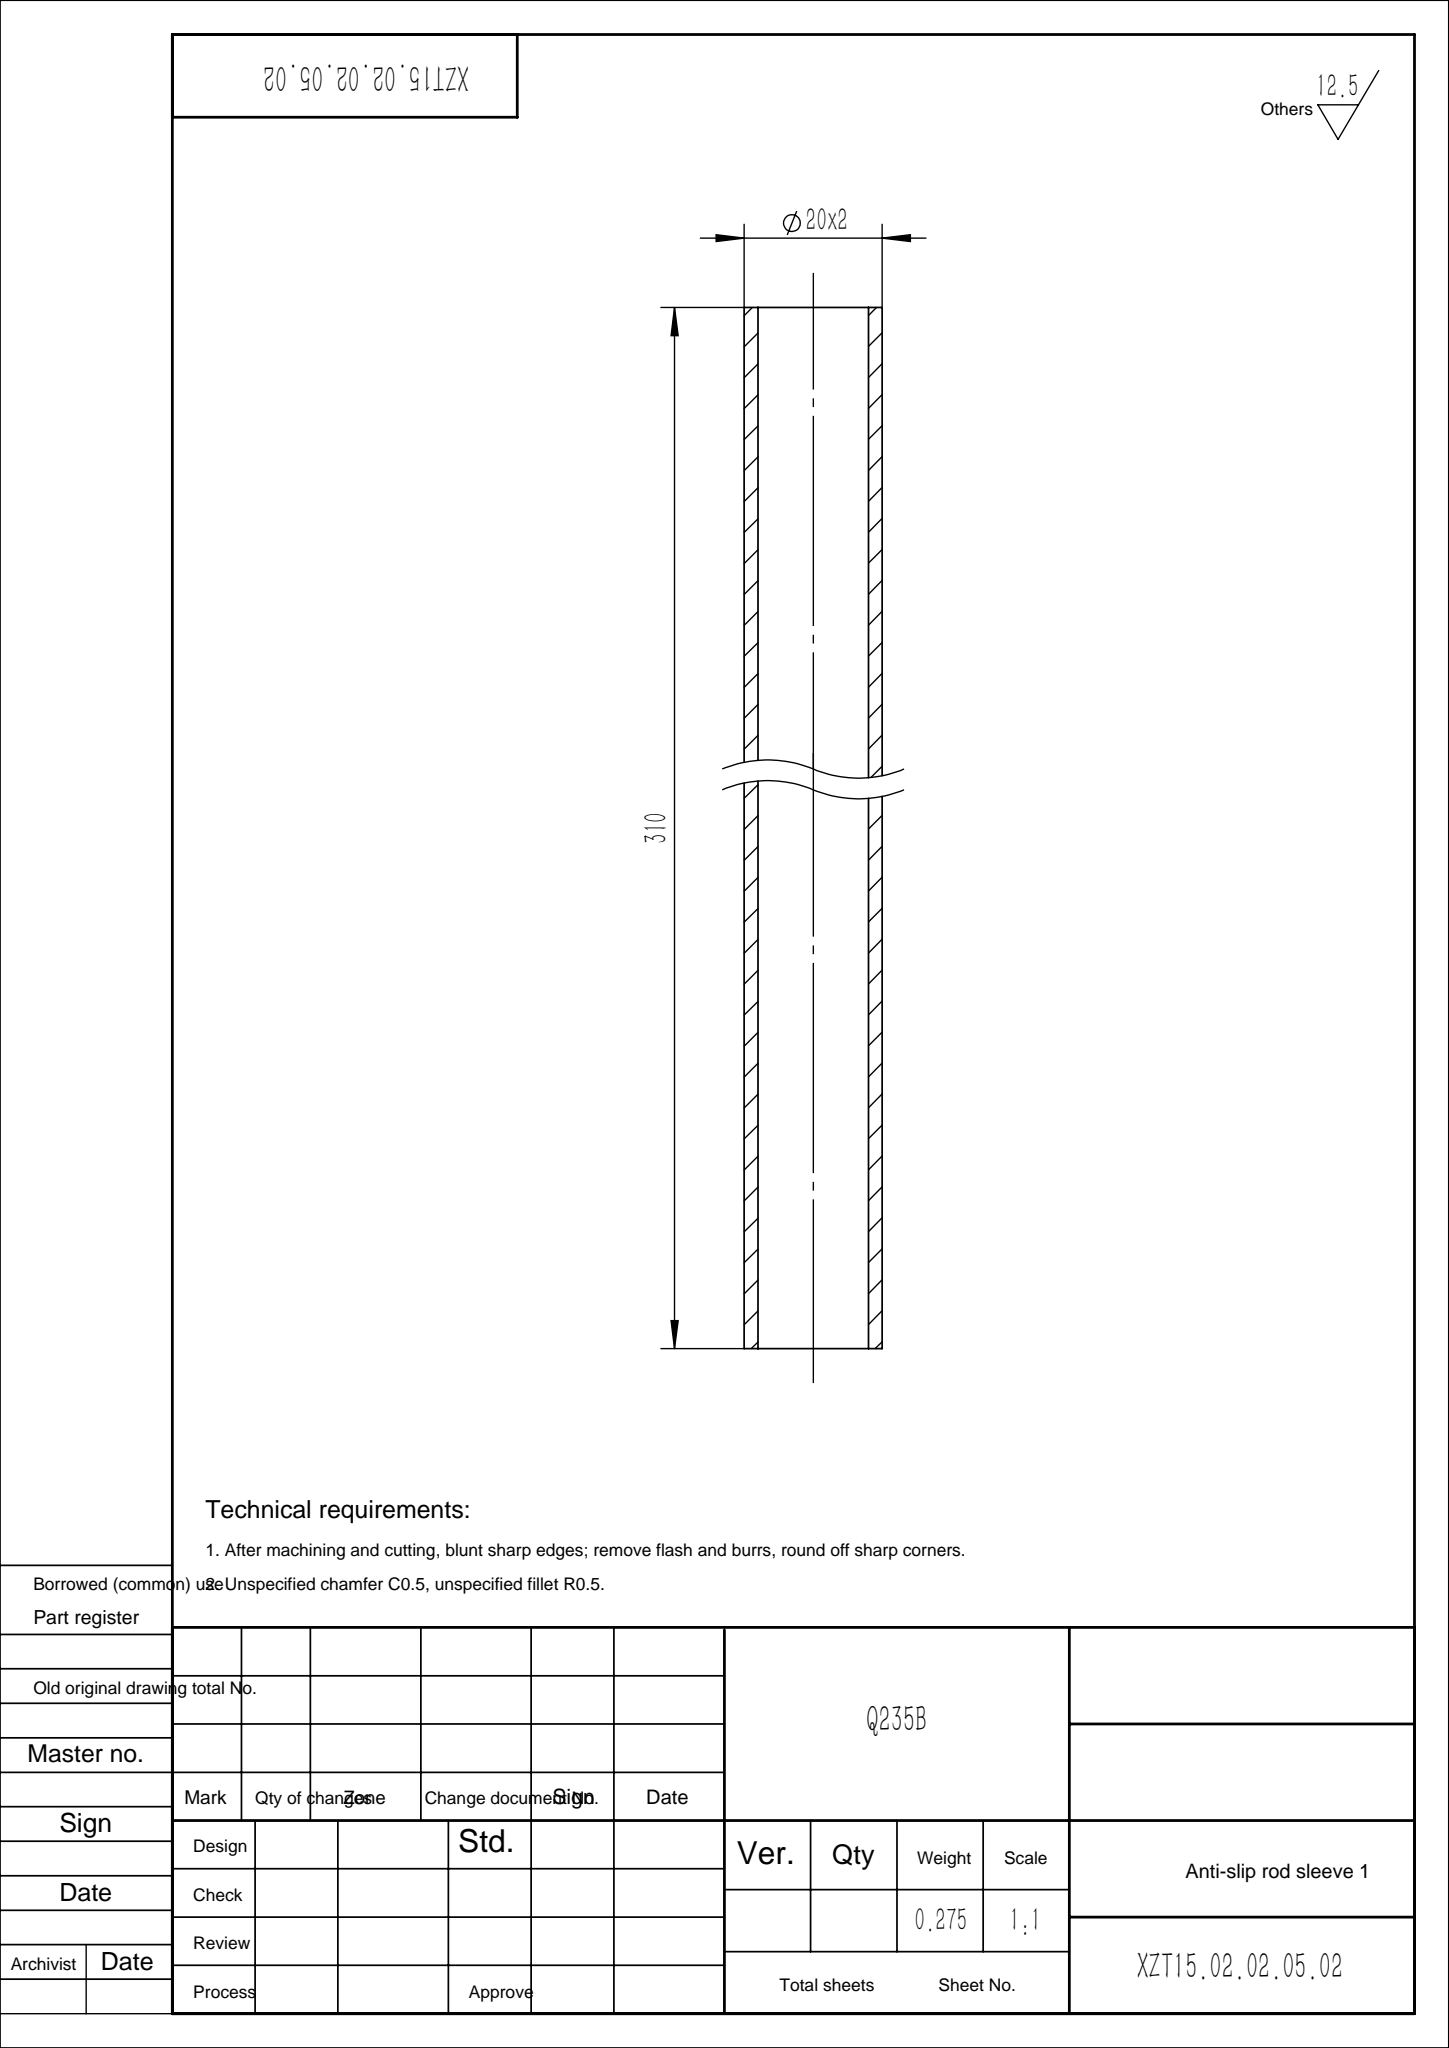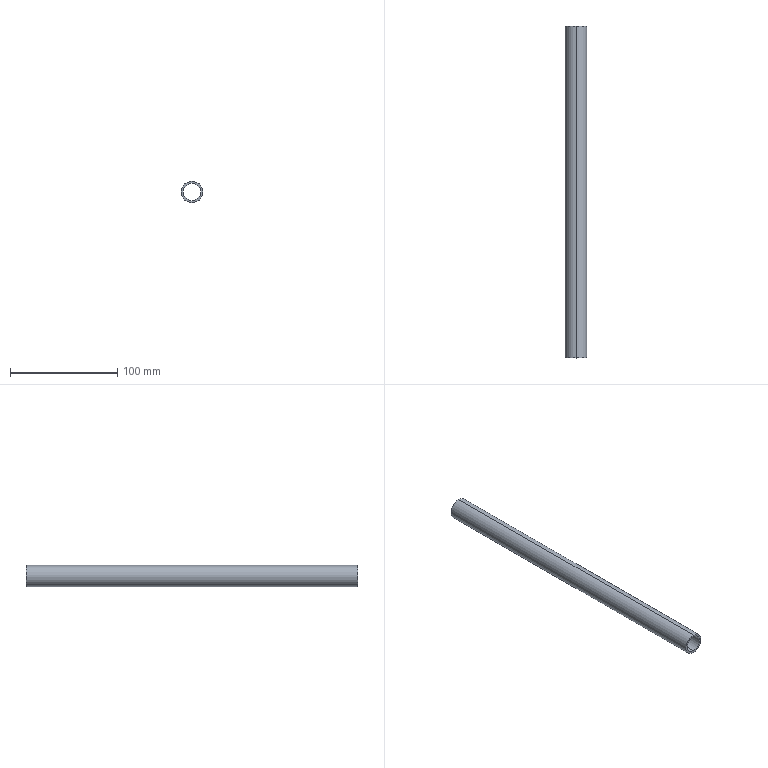Part | SolidWorks | features WeldMemberFeat 1, WeldmentFeature 1 | 1 solid | 6 faces | box 20 x 310 x 20 mm | volume 35060 mm3 | cylinder 4 | plane 2 | commonest cylinder face diameters 16 x2 20 x2
STEP:
#1=CARTESIAN_POINT('',(0.,310.,10.));
#2=VERTEX_POINT('',#1);
#3=CARTESIAN_POINT('',(0.,310.,-10.));
#4=VERTEX_POINT('',#3);
#5=CARTESIAN_POINT('',(0.,310.,0.));
#6=DIRECTION('',(0.,1.,0.));
#7=DIRECTION('',(0.,0.,1.));
#8=AXIS2_PLACEMENT_3D('',#5,#6,#7);
#9=CIRCLE('',#8,10.);
#10=EDGE_CURVE('',#2,#4,#9,.T.);
#11=ORIENTED_EDGE('',*,*,#10,.F.);
#12=CARTESIAN_POINT('',(0.,0.,10.));
#13=VERTEX_POINT('',#12);
#14=CARTESIAN_POINT('',(0.,310.,10.));
#15=DIRECTION('',(0.,-1.,0.));
#16=VECTOR('',#15,1000.);
#17=LINE('',#14,#16);
#18=EDGE_CURVE('',#2,#13,#17,.T.);
#19=ORIENTED_EDGE('',*,*,#18,.T.);
#20=CARTESIAN_POINT('',(0.,0.,-10.));
#21=VERTEX_POINT('',#20);
#22=CARTESIAN_POINT('',(0.,0.,0.));
#23=DIRECTION('',(0.,1.,0.));
#24=DIRECTION('',(0.,0.,1.));
#25=AXIS2_PLACEMENT_3D('',#22,#23,#24);
#26=CIRCLE('',#25,10.);
#27=EDGE_CURVE('',#13,#21,#26,.T.);
#28=ORIENTED_EDGE('',*,*,#27,.T.);
#29=CARTESIAN_POINT('',(0.,310.,-10.));
#30=DIRECTION('',(0.,-1.,0.));
#31=VECTOR('',#30,1000.);
#32=LINE('',#29,#31);
#33=EDGE_CURVE('',#4,#21,#32,.T.);
#34=ORIENTED_EDGE('',*,*,#33,.F.);
#35=EDGE_LOOP('',(#11,#19,#28,#34));
#36=FACE_OUTER_BOUND('',#35,.T.);
#37=CARTESIAN_POINT('',(0.,310.,0.));
#38=DIRECTION('',(0.,-1.,0.));
#39=DIRECTION('',(0.,0.,-1.));
#40=AXIS2_PLACEMENT_3D('',#37,#38,#39);
#41=CYLINDRICAL_SURFACE('',#40,10.);
#42=ADVANCED_FACE('',(#36),#41,.T.);
#43=CARTESIAN_POINT('',(0.,310.,-8.));
#44=VERTEX_POINT('',#43);
#45=CARTESIAN_POINT('',(0.,310.,8.));
#46=VERTEX_POINT('',#45);
#47=CARTESIAN_POINT('',(0.,310.,0.));
#48=DIRECTION('',(0.,1.,0.));
#49=DIRECTION('',(0.,0.,1.));
#50=AXIS2_PLACEMENT_3D('',#47,#48,#49);
#51=CIRCLE('',#50,8.);
#52=EDGE_CURVE('',#44,#46,#51,.T.);
#53=ORIENTED_EDGE('',*,*,#52,.T.);
#54=CARTESIAN_POINT('',(0.,0.,8.));
#55=VERTEX_POINT('',#54);
#56=CARTESIAN_POINT('',(0.,310.,8.));
#57=DIRECTION('',(0.,-1.,0.));
#58=VECTOR('',#57,1000.);
#59=LINE('',#56,#58);
#60=EDGE_CURVE('',#46,#55,#59,.T.);
#61=ORIENTED_EDGE('',*,*,#60,.T.);
#62=CARTESIAN_POINT('',(0.,0.,-8.));
#63=VERTEX_POINT('',#62);
#64=CARTESIAN_POINT('',(0.,0.,0.));
#65=DIRECTION('',(0.,1.,0.));
#66=DIRECTION('',(0.,0.,1.));
#67=AXIS2_PLACEMENT_3D('',#64,#65,#66);
#68=CIRCLE('',#67,8.);
#69=EDGE_CURVE('',#63,#55,#68,.T.);
#70=ORIENTED_EDGE('',*,*,#69,.F.);
#71=CARTESIAN_POINT('',(0.,310.,-8.));
#72=DIRECTION('',(0.,-1.,0.));
#73=VECTOR('',#72,1000.);
#74=LINE('',#71,#73);
#75=EDGE_CURVE('',#44,#63,#74,.T.);
#76=ORIENTED_EDGE('',*,*,#75,.F.);
#77=EDGE_LOOP('',(#53,#61,#70,#76));
#78=FACE_OUTER_BOUND('',#77,.T.);
#79=CARTESIAN_POINT('',(0.,310.,0.));
#80=DIRECTION('',(0.,-1.,0.));
#81=DIRECTION('',(0.,0.,-1.));
#82=AXIS2_PLACEMENT_3D('',#79,#80,#81);
#83=CYLINDRICAL_SURFACE('',#82,8.);
#84=ADVANCED_FACE('',(#78),#83,.F.);
#85=ORIENTED_EDGE('',*,*,#60,.F.);
#86=CARTESIAN_POINT('',(0.,310.,0.));
#87=DIRECTION('',(0.,1.,0.));
#88=DIRECTION('',(0.,0.,1.));
#89=AXIS2_PLACEMENT_3D('',#86,#87,#88);
#90=CIRCLE('',#89,8.);
#91=EDGE_CURVE('',#46,#44,#90,.T.);
#92=ORIENTED_EDGE('',*,*,#91,.T.);
#93=ORIENTED_EDGE('',*,*,#75,.T.);
#94=CARTESIAN_POINT('',(0.,0.,0.));
#95=DIRECTION('',(0.,1.,0.));
#96=DIRECTION('',(0.,0.,1.));
#97=AXIS2_PLACEMENT_3D('',#94,#95,#96);
#98=CIRCLE('',#97,8.);
#99=EDGE_CURVE('',#55,#63,#98,.T.);
#100=ORIENTED_EDGE('',*,*,#99,.F.);
#101=EDGE_LOOP('',(#85,#92,#93,#100));
#102=FACE_OUTER_BOUND('',#101,.T.);
#103=CARTESIAN_POINT('',(0.,310.,0.));
#104=DIRECTION('',(0.,-1.,0.));
#105=DIRECTION('',(0.,0.,-1.));
#106=AXIS2_PLACEMENT_3D('',#103,#104,#105);
#107=CYLINDRICAL_SURFACE('',#106,8.);
#108=ADVANCED_FACE('',(#102),#107,.F.);
#109=ORIENTED_EDGE('',*,*,#18,.F.);
#110=CARTESIAN_POINT('',(0.,310.,0.));
#111=DIRECTION('',(0.,1.,0.));
#112=DIRECTION('',(0.,0.,1.));
#113=AXIS2_PLACEMENT_3D('',#110,#111,#112);
#114=CIRCLE('',#113,10.);
#115=EDGE_CURVE('',#4,#2,#114,.T.);
#116=ORIENTED_EDGE('',*,*,#115,.F.);
#117=ORIENTED_EDGE('',*,*,#33,.T.);
#118=CARTESIAN_POINT('',(0.,0.,0.));
#119=DIRECTION('',(0.,1.,0.));
#120=DIRECTION('',(0.,0.,1.));
#121=AXIS2_PLACEMENT_3D('',#118,#119,#120);
#122=CIRCLE('',#121,10.);
#123=EDGE_CURVE('',#21,#13,#122,.T.);
#124=ORIENTED_EDGE('',*,*,#123,.T.);
#125=EDGE_LOOP('',(#109,#116,#117,#124));
#126=FACE_OUTER_BOUND('',#125,.T.);
#127=CARTESIAN_POINT('',(0.,310.,0.));
#128=DIRECTION('',(0.,-1.,0.));
#129=DIRECTION('',(0.,0.,-1.));
#130=AXIS2_PLACEMENT_3D('',#127,#128,#129);
#131=CYLINDRICAL_SURFACE('',#130,10.);
#132=ADVANCED_FACE('',(#126),#131,.T.);
#133=ORIENTED_EDGE('',*,*,#52,.F.);
#134=ORIENTED_EDGE('',*,*,#91,.F.);
#135=EDGE_LOOP('',(#133,#134));
#136=FACE_BOUND('',#135,.T.);
#137=ORIENTED_EDGE('',*,*,#115,.T.);
#138=ORIENTED_EDGE('',*,*,#10,.T.);
#139=EDGE_LOOP('',(#137,#138));
#140=FACE_OUTER_BOUND('',#139,.T.);
#141=CARTESIAN_POINT('',(0.,310.,0.));
#142=DIRECTION('',(0.,1.,0.));
#143=DIRECTION('',(0.,0.,1.));
#144=AXIS2_PLACEMENT_3D('',#141,#142,#143);
#145=PLANE('',#144);
#146=ADVANCED_FACE('',(#136,#140),#145,.T.);
#147=ORIENTED_EDGE('',*,*,#69,.T.);
#148=ORIENTED_EDGE('',*,*,#99,.T.);
#149=EDGE_LOOP('',(#147,#148));
#150=FACE_BOUND('',#149,.T.);
#151=ORIENTED_EDGE('',*,*,#123,.F.);
#152=ORIENTED_EDGE('',*,*,#27,.F.);
#153=EDGE_LOOP('',(#151,#152));
#154=FACE_OUTER_BOUND('',#153,.T.);
#155=CARTESIAN_POINT('',(0.,0.,0.));
#156=DIRECTION('',(0.,1.,0.));
#157=DIRECTION('',(0.,0.,1.));
#158=AXIS2_PLACEMENT_3D('',#155,#156,#157);
#159=PLANE('',#158);
#160=ADVANCED_FACE('',(#150,#154),#159,.F.);
#161=CLOSED_SHELL('',(#42,#84,#108,#132,#146,#160));
#162=MANIFOLD_SOLID_BREP('',#161);
#163=CARTESIAN_POINT('',(0.,0.,0.));
#164=DIRECTION('',(0.,0.,1.));
#165=DIRECTION('',(1.,0.,0.));
#166=AXIS2_PLACEMENT_3D('',#163,#164,#165);
#167=(LENGTH_UNIT()NAMED_UNIT(*)SI_UNIT(.MILLI.,.METRE.));
#168=UNCERTAINTY_MEASURE_WITH_UNIT(LENGTH_MEASURE(0.00001),#167,'','');
#169=(NAMED_UNIT(*)PLANE_ANGLE_UNIT()SI_UNIT($,.RADIAN.));
#170=(NAMED_UNIT(*)SI_UNIT($,.STERADIAN.)SOLID_ANGLE_UNIT());
#171=(GEOMETRIC_REPRESENTATION_CONTEXT(3)GLOBAL_UNCERTAINTY_ASSIGNED_CONTEXT((#168))GLOBAL_UNIT_ASSIGNED_CONTEXT((#167,#169,#170))REPRESENTATION_CONTEXT('',''));
#172=ADVANCED_BREP_SHAPE_REPRESENTATION('',(#162,#166),#171);